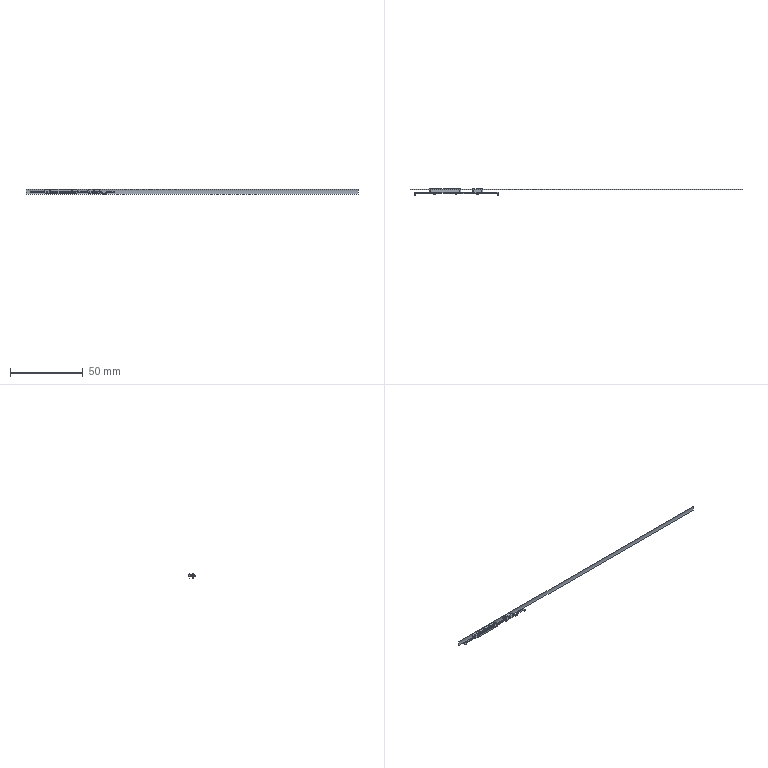Part | Creo | 1 solid | 98 faces | box 228.88 x 4.8 x 3.7 mm | volume 376.003 mm3 | plane 50 | cylinder 36 | torus 6 | spline 4 | cone 2 | commonest cylinder face diameters 1.2 x6 12.412 x5 0.6 x4 0.75 x4 1.75 x4 2.95 x4